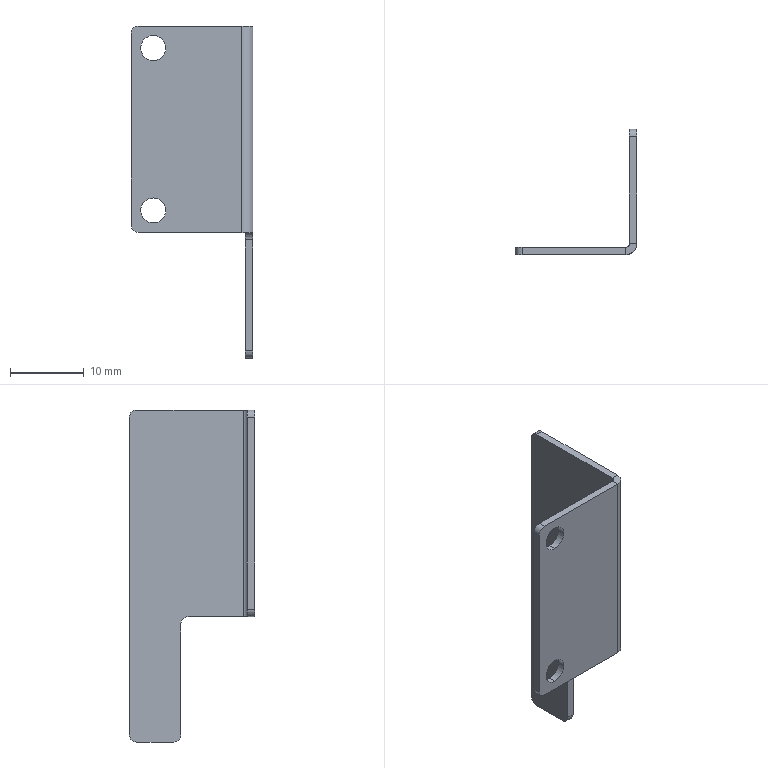Part | NX | features BREP 1 | 1 solid | 26 faces | box 16.5 x 17 x 45 mm | volume 997.965 mm3 | plane 14 | cylinder 12 | commonest cylinder face diameters 2 x6 3.4 x4 1 x1 3 x1
STEP:
#1=CARTESIAN_POINT('',(-12.5,-16.,17.8));
#2=VERTEX_POINT('',#1);
#3=CARTESIAN_POINT('',(-12.5,-17.,17.8));
#4=VERTEX_POINT('',#3);
#5=CARTESIAN_POINT('',(-12.5,-16.,17.8));
#6=DIRECTION('',(0.,1.,0.));
#7=VECTOR('',#6,1000.);
#8=LINE('',#5,#7);
#9=EDGE_CURVE('',#2,#4,#8,.F.);
#10=ORIENTED_EDGE('',*,*,#9,.T.);
#11=CARTESIAN_POINT('',(-12.5,-17.,21.2));
#12=VERTEX_POINT('',#11);
#13=CARTESIAN_POINT('',(-12.5,-17.,19.5));
#14=DIRECTION('',(0.,1.,0.));
#15=DIRECTION('',(0.,0.,1.));
#16=AXIS2_PLACEMENT_3D('',#13,#14,#15);
#17=CIRCLE('',#16,1.7);
#18=EDGE_CURVE('',#12,#4,#17,.T.);
#19=ORIENTED_EDGE('',*,*,#18,.F.);
#20=CARTESIAN_POINT('',(-12.5,-16.,21.2));
#21=VERTEX_POINT('',#20);
#22=CARTESIAN_POINT('',(-12.5,-16.,21.2));
#23=DIRECTION('',(0.,1.,0.));
#24=VECTOR('',#23,1000.);
#25=LINE('',#22,#24);
#26=EDGE_CURVE('',#21,#12,#25,.F.);
#27=ORIENTED_EDGE('',*,*,#26,.F.);
#28=CARTESIAN_POINT('',(-12.5,-16.,19.5));
#29=DIRECTION('',(0.,1.,0.));
#30=DIRECTION('',(0.,0.,1.));
#31=AXIS2_PLACEMENT_3D('',#28,#29,#30);
#32=CIRCLE('',#31,1.7);
#33=EDGE_CURVE('',#21,#2,#32,.T.);
#34=ORIENTED_EDGE('',*,*,#33,.T.);
#35=EDGE_LOOP('',(#10,#19,#27,#34));
#36=FACE_BOUND('',#35,.T.);
#37=CARTESIAN_POINT('',(-12.5,-16.,19.5));
#38=DIRECTION('',(0.,1.,0.));
#39=DIRECTION('',(0.,0.,1.));
#40=AXIS2_PLACEMENT_3D('',#37,#38,#39);
#41=CYLINDRICAL_SURFACE('',#40,1.7);
#42=ADVANCED_FACE('',(#36),#41,.F.);
#43=CARTESIAN_POINT('',(-12.5,-16.,-4.2));
#44=VERTEX_POINT('',#43);
#45=CARTESIAN_POINT('',(-12.5,-17.,-4.2));
#46=VERTEX_POINT('',#45);
#47=CARTESIAN_POINT('',(-12.5,-16.,-4.2));
#48=DIRECTION('',(0.,1.,0.));
#49=VECTOR('',#48,1000.);
#50=LINE('',#47,#49);
#51=EDGE_CURVE('',#44,#46,#50,.F.);
#52=ORIENTED_EDGE('',*,*,#51,.T.);
#53=CARTESIAN_POINT('',(-12.5,-17.,-0.8));
#54=VERTEX_POINT('',#53);
#55=CARTESIAN_POINT('',(-12.5,-17.,-2.5));
#56=DIRECTION('',(0.,1.,0.));
#57=DIRECTION('',(0.,0.,1.));
#58=AXIS2_PLACEMENT_3D('',#55,#56,#57);
#59=CIRCLE('',#58,1.7);
#60=EDGE_CURVE('',#54,#46,#59,.T.);
#61=ORIENTED_EDGE('',*,*,#60,.F.);
#62=CARTESIAN_POINT('',(-12.5,-16.,-0.8));
#63=VERTEX_POINT('',#62);
#64=CARTESIAN_POINT('',(-12.5,-16.,-0.8));
#65=DIRECTION('',(0.,1.,0.));
#66=VECTOR('',#65,1000.);
#67=LINE('',#64,#66);
#68=EDGE_CURVE('',#63,#54,#67,.F.);
#69=ORIENTED_EDGE('',*,*,#68,.F.);
#70=CARTESIAN_POINT('',(-12.5,-16.,-2.5));
#71=DIRECTION('',(0.,1.,0.));
#72=DIRECTION('',(0.,0.,1.));
#73=AXIS2_PLACEMENT_3D('',#70,#71,#72);
#74=CIRCLE('',#73,1.7);
#75=EDGE_CURVE('',#63,#44,#74,.T.);
#76=ORIENTED_EDGE('',*,*,#75,.T.);
#77=EDGE_LOOP('',(#52,#61,#69,#76));
#78=FACE_BOUND('',#77,.T.);
#79=CARTESIAN_POINT('',(-12.5,-16.,-2.5));
#80=DIRECTION('',(0.,1.,0.));
#81=DIRECTION('',(0.,0.,1.));
#82=AXIS2_PLACEMENT_3D('',#79,#80,#81);
#83=CYLINDRICAL_SURFACE('',#82,1.7);
#84=ADVANCED_FACE('',(#78),#83,.F.);
#85=CARTESIAN_POINT('',(-14.5,-17.,22.5));
#86=VERTEX_POINT('',#85);
#87=CARTESIAN_POINT('',(-15.5,-17.,21.5));
#88=VERTEX_POINT('',#87);
#89=CARTESIAN_POINT('',(-14.5,-17.,21.5));
#90=DIRECTION('',(0.,-1.,0.));
#91=DIRECTION('',(-1.,0.,0.));
#92=AXIS2_PLACEMENT_3D('',#89,#90,#91);
#93=CIRCLE('',#92,1.);
#94=EDGE_CURVE('',#86,#88,#93,.T.);
#95=ORIENTED_EDGE('',*,*,#94,.F.);
#96=CARTESIAN_POINT('',(-14.5,-16.,22.5));
#97=VERTEX_POINT('',#96);
#98=CARTESIAN_POINT('',(-14.5,-15.5,22.5));
#99=DIRECTION('',(0.,-1.,0.));
#100=VECTOR('',#99,1000.);
#101=LINE('',#98,#100);
#102=EDGE_CURVE('',#97,#86,#101,.T.);
#103=ORIENTED_EDGE('',*,*,#102,.F.);
#104=CARTESIAN_POINT('',(-15.5,-16.,21.5));
#105=VERTEX_POINT('',#104);
#106=CARTESIAN_POINT('',(-14.5,-16.,21.5));
#107=DIRECTION('',(0.,1.,0.));
#108=DIRECTION('',(-1.,0.,0.));
#109=AXIS2_PLACEMENT_3D('',#106,#107,#108);
#110=CIRCLE('',#109,1.);
#111=EDGE_CURVE('',#105,#97,#110,.T.);
#112=ORIENTED_EDGE('',*,*,#111,.F.);
#113=CARTESIAN_POINT('',(-15.5,-17.,21.5));
#114=DIRECTION('',(0.,1.,0.));
#115=VECTOR('',#114,1000.);
#116=LINE('',#113,#115);
#117=EDGE_CURVE('',#88,#105,#116,.T.);
#118=ORIENTED_EDGE('',*,*,#117,.F.);
#119=EDGE_LOOP('',(#95,#103,#112,#118));
#120=FACE_BOUND('',#119,.T.);
#121=CARTESIAN_POINT('',(-14.5,-17.,21.5));
#122=DIRECTION('',(0.,1.,0.));
#123=DIRECTION('',(0.,0.,1.));
#124=AXIS2_PLACEMENT_3D('',#121,#122,#123);
#125=CYLINDRICAL_SURFACE('',#124,1.);
#126=ADVANCED_FACE('',(#120),#125,.T.);
#127=CARTESIAN_POINT('',(-14.5,-16.,-5.5));
#128=VERTEX_POINT('',#127);
#129=CARTESIAN_POINT('',(-15.5,-16.,-4.5));
#130=VERTEX_POINT('',#129);
#131=CARTESIAN_POINT('',(-14.5,-16.,-4.5));
#132=DIRECTION('',(0.,1.,0.));
#133=DIRECTION('',(-1.,0.,0.));
#134=AXIS2_PLACEMENT_3D('',#131,#132,#133);
#135=CIRCLE('',#134,1.);
#136=EDGE_CURVE('',#128,#130,#135,.T.);
#137=ORIENTED_EDGE('',*,*,#136,.F.);
#138=CARTESIAN_POINT('',(-14.5,-17.,-5.5));
#139=VERTEX_POINT('',#138);
#140=CARTESIAN_POINT('',(-14.5,-16.,-5.5));
#141=DIRECTION('',(0.,1.,0.));
#142=VECTOR('',#141,1000.);
#143=LINE('',#140,#142);
#144=EDGE_CURVE('',#139,#128,#143,.T.);
#145=ORIENTED_EDGE('',*,*,#144,.F.);
#146=CARTESIAN_POINT('',(-15.5,-17.,-4.5));
#147=VERTEX_POINT('',#146);
#148=CARTESIAN_POINT('',(-14.5,-17.,-4.5));
#149=DIRECTION('',(0.,-1.,0.));
#150=DIRECTION('',(-1.,0.,0.));
#151=AXIS2_PLACEMENT_3D('',#148,#149,#150);
#152=CIRCLE('',#151,1.);
#153=EDGE_CURVE('',#147,#139,#152,.T.);
#154=ORIENTED_EDGE('',*,*,#153,.F.);
#155=CARTESIAN_POINT('',(-15.5,-17.,-4.5));
#156=DIRECTION('',(0.,-1.,0.));
#157=VECTOR('',#156,1000.);
#158=LINE('',#155,#157);
#159=EDGE_CURVE('',#130,#147,#158,.T.);
#160=ORIENTED_EDGE('',*,*,#159,.F.);
#161=EDGE_LOOP('',(#137,#145,#154,#160));
#162=FACE_BOUND('',#161,.T.);
#163=CARTESIAN_POINT('',(-14.5,-17.,-4.5));
#164=DIRECTION('',(0.,1.,0.));
#165=DIRECTION('',(0.,0.,1.));
#166=AXIS2_PLACEMENT_3D('',#163,#164,#165);
#167=CYLINDRICAL_SURFACE('',#166,1.);
#168=ADVANCED_FACE('',(#162),#167,.T.);
#169=CARTESIAN_POINT('',(0.,-1.,22.5));
#170=VERTEX_POINT('',#169);
#171=CARTESIAN_POINT('',(0.,0.,21.5));
#172=VERTEX_POINT('',#171);
#173=CARTESIAN_POINT('',(0.,-1.,21.5));
#174=DIRECTION('',(-1.,0.,0.));
#175=DIRECTION('',(0.,-1.,0.));
#176=AXIS2_PLACEMENT_3D('',#173,#174,#175);
#177=CIRCLE('',#176,1.);
#178=EDGE_CURVE('',#170,#172,#177,.T.);
#179=ORIENTED_EDGE('',*,*,#178,.F.);
#180=CARTESIAN_POINT('',(1.,-1.,22.5));
#181=VERTEX_POINT('',#180);
#182=CARTESIAN_POINT('',(-0.5,-1.,22.5));
#183=DIRECTION('',(-1.,0.,0.));
#184=VECTOR('',#183,1000.);
#185=LINE('',#182,#184);
#186=EDGE_CURVE('',#181,#170,#185,.T.);
#187=ORIENTED_EDGE('',*,*,#186,.F.);
#188=CARTESIAN_POINT('',(1.,0.,21.5));
#189=VERTEX_POINT('',#188);
#190=CARTESIAN_POINT('',(1.,-1.,21.5));
#191=DIRECTION('',(1.,0.,0.));
#192=DIRECTION('',(0.,-1.,0.));
#193=AXIS2_PLACEMENT_3D('',#190,#191,#192);
#194=CIRCLE('',#193,1.);
#195=EDGE_CURVE('',#189,#181,#194,.T.);
#196=ORIENTED_EDGE('',*,*,#195,.F.);
#197=CARTESIAN_POINT('',(0.,0.,21.5));
#198=DIRECTION('',(1.,0.,0.));
#199=VECTOR('',#198,1000.);
#200=LINE('',#197,#199);
#201=EDGE_CURVE('',#172,#189,#200,.T.);
#202=ORIENTED_EDGE('',*,*,#201,.F.);
#203=EDGE_LOOP('',(#179,#187,#196,#202));
#204=FACE_BOUND('',#203,.T.);
#205=CARTESIAN_POINT('',(0.,-1.,21.5));
#206=DIRECTION('',(1.,0.,0.));
#207=DIRECTION('',(0.,1.,0.));
#208=AXIS2_PLACEMENT_3D('',#205,#206,#207);
#209=CYLINDRICAL_SURFACE('',#208,1.);
#210=ADVANCED_FACE('',(#204),#209,.T.);
#211=CARTESIAN_POINT('',(0.,-7.,-6.5));
#212=VERTEX_POINT('',#211);
#213=CARTESIAN_POINT('',(0.,-8.,-5.5));
#214=VERTEX_POINT('',#213);
#215=CARTESIAN_POINT('',(0.,-8.,-6.5));
#216=DIRECTION('',(1.,0.,0.));
#217=DIRECTION('',(0.,-1.,0.));
#218=AXIS2_PLACEMENT_3D('',#215,#216,#217);
#219=CIRCLE('',#218,1.);
#220=EDGE_CURVE('',#212,#214,#219,.T.);
#221=ORIENTED_EDGE('',*,*,#220,.F.);
#222=CARTESIAN_POINT('',(1.,-7.,-6.5));
#223=VERTEX_POINT('',#222);
#224=CARTESIAN_POINT('',(0.,-7.,-6.5));
#225=DIRECTION('',(-1.,0.,0.));
#226=VECTOR('',#225,1000.);
#227=LINE('',#224,#226);
#228=EDGE_CURVE('',#223,#212,#227,.T.);
#229=ORIENTED_EDGE('',*,*,#228,.F.);
#230=CARTESIAN_POINT('',(1.,-8.,-5.5));
#231=VERTEX_POINT('',#230);
#232=CARTESIAN_POINT('',(1.,-8.,-6.5));
#233=DIRECTION('',(-1.,0.,0.));
#234=DIRECTION('',(0.,-1.,0.));
#235=AXIS2_PLACEMENT_3D('',#232,#233,#234);
#236=CIRCLE('',#235,1.);
#237=EDGE_CURVE('',#231,#223,#236,.T.);
#238=ORIENTED_EDGE('',*,*,#237,.F.);
#239=CARTESIAN_POINT('',(1.,-8.,-5.5));
#240=DIRECTION('',(1.,0.,0.));
#241=VECTOR('',#240,1000.);
#242=LINE('',#239,#241);
#243=EDGE_CURVE('',#214,#231,#242,.T.);
#244=ORIENTED_EDGE('',*,*,#243,.F.);
#245=EDGE_LOOP('',(#221,#229,#238,#244));
#246=FACE_BOUND('',#245,.T.);
#247=CARTESIAN_POINT('',(-15.5,-8.,-6.5));
#248=DIRECTION('',(-1.,0.,0.));
#249=DIRECTION('',(0.,-1.,0.));
#250=AXIS2_PLACEMENT_3D('',#247,#248,#249);
#251=CYLINDRICAL_SURFACE('',#250,1.);
#252=ADVANCED_FACE('',(#246),#251,.F.);
#253=CARTESIAN_POINT('',(0.,0.,-21.5));
#254=VERTEX_POINT('',#253);
#255=CARTESIAN_POINT('',(0.,-1.,-22.5));
#256=VERTEX_POINT('',#255);
#257=CARTESIAN_POINT('',(0.,-1.,-21.5));
#258=DIRECTION('',(-1.,0.,0.));
#259=DIRECTION('',(0.,-1.,0.));
#260=AXIS2_PLACEMENT_3D('',#257,#258,#259);
#261=CIRCLE('',#260,1.);
#262=EDGE_CURVE('',#254,#256,#261,.T.);
#263=ORIENTED_EDGE('',*,*,#262,.F.);
#264=CARTESIAN_POINT('',(1.,0.,-21.5));
#265=VERTEX_POINT('',#264);
#266=CARTESIAN_POINT('',(0.,0.,-21.5));
#267=DIRECTION('',(-1.,0.,0.));
#268=VECTOR('',#267,1000.);
#269=LINE('',#266,#268);
#270=EDGE_CURVE('',#265,#254,#269,.T.);
#271=ORIENTED_EDGE('',*,*,#270,.F.);
#272=CARTESIAN_POINT('',(1.,-1.,-22.5));
#273=VERTEX_POINT('',#272);
#274=CARTESIAN_POINT('',(1.,-1.,-21.5));
#275=DIRECTION('',(1.,0.,0.));
#276=DIRECTION('',(0.,-1.,0.));
#277=AXIS2_PLACEMENT_3D('',#274,#275,#276);
#278=CIRCLE('',#277,1.);
#279=EDGE_CURVE('',#273,#265,#278,.T.);
#280=ORIENTED_EDGE('',*,*,#279,.F.);
#281=CARTESIAN_POINT('',(1.,-1.,-22.5));
#282=DIRECTION('',(1.,0.,0.));
#283=VECTOR('',#282,1000.);
#284=LINE('',#281,#283);
#285=EDGE_CURVE('',#256,#273,#284,.T.);
#286=ORIENTED_EDGE('',*,*,#285,.F.);
#287=EDGE_LOOP('',(#263,#271,#280,#286));
#288=FACE_BOUND('',#287,.T.);
#289=CARTESIAN_POINT('',(-0.5,-1.,-21.5));
#290=DIRECTION('',(-1.,0.,0.));
#291=DIRECTION('',(0.,-1.,0.));
#292=AXIS2_PLACEMENT_3D('',#289,#290,#291);
#293=CYLINDRICAL_SURFACE('',#292,1.);
#294=ADVANCED_FACE('',(#288),#293,.T.);
#295=CARTESIAN_POINT('',(1.,-7.,-21.5));
#296=VERTEX_POINT('',#295);
#297=CARTESIAN_POINT('',(1.,-6.,-22.5));
#298=VERTEX_POINT('',#297);
#299=CARTESIAN_POINT('',(1.,-6.,-21.5));
#300=DIRECTION('',(1.,0.,0.));
#301=DIRECTION('',(0.,-1.,0.));
#302=AXIS2_PLACEMENT_3D('',#299,#300,#301);
#303=CIRCLE('',#302,1.);
#304=EDGE_CURVE('',#296,#298,#303,.T.);
#305=ORIENTED_EDGE('',*,*,#304,.F.);
#306=CARTESIAN_POINT('',(0.,-7.,-21.5));
#307=VERTEX_POINT('',#306);
#308=CARTESIAN_POINT('',(-15.5,-7.,-21.5));
#309=DIRECTION('',(1.,0.,0.));
#310=VECTOR('',#309,1000.);
#311=LINE('',#308,#310);
#312=EDGE_CURVE('',#307,#296,#311,.T.);
#313=ORIENTED_EDGE('',*,*,#312,.F.);
#314=CARTESIAN_POINT('',(0.,-6.,-22.5));
#315=VERTEX_POINT('',#314);
#316=CARTESIAN_POINT('',(0.,-6.,-21.5));
#317=DIRECTION('',(-1.,0.,0.));
#318=DIRECTION('',(0.,-1.,0.));
#319=AXIS2_PLACEMENT_3D('',#316,#317,#318);
#320=CIRCLE('',#319,1.);
#321=EDGE_CURVE('',#315,#307,#320,.T.);
#322=ORIENTED_EDGE('',*,*,#321,.F.);
#323=CARTESIAN_POINT('',(-0.5,-6.,-22.5));
#324=DIRECTION('',(-1.,0.,0.));
#325=VECTOR('',#324,1000.);
#326=LINE('',#323,#325);
#327=EDGE_CURVE('',#298,#315,#326,.T.);
#328=ORIENTED_EDGE('',*,*,#327,.F.);
#329=EDGE_LOOP('',(#305,#313,#322,#328));
#330=FACE_BOUND('',#329,.T.);
#331=CARTESIAN_POINT('',(-0.5,-6.,-21.5));
#332=DIRECTION('',(-1.,0.,0.));
#333=DIRECTION('',(0.,-1.,0.));
#334=AXIS2_PLACEMENT_3D('',#331,#332,#333);
#335=CYLINDRICAL_SURFACE('',#334,1.);
#336=ADVANCED_FACE('',(#330),#335,.T.);
#337=CARTESIAN_POINT('',(0.,-7.,22.5));
#338=DIRECTION('',(0.,0.,-1.));
#339=VECTOR('',#338,1000.);
#340=LINE('',#337,#339);
#341=EDGE_CURVE('',#212,#307,#340,.T.);
#342=ORIENTED_EDGE('',*,*,#341,.T.);
#343=ORIENTED_EDGE('',*,*,#312,.T.);
#344=CARTESIAN_POINT('',(1.,-7.,-22.5));
#345=DIRECTION('',(0.,0.,1.));
#346=VECTOR('',#345,1000.);
#347=LINE('',#344,#346);
#348=EDGE_CURVE('',#296,#223,#347,.T.);
#349=ORIENTED_EDGE('',*,*,#348,.T.);
#350=ORIENTED_EDGE('',*,*,#228,.T.);
#351=EDGE_LOOP('',(#342,#343,#349,#350));
#352=FACE_BOUND('',#351,.T.);
#353=CARTESIAN_POINT('',(-15.5,-7.,-22.5));
#354=DIRECTION('',(0.,1.,0.));
#355=DIRECTION('',(-1.,0.,0.));
#356=AXIS2_PLACEMENT_3D('',#353,#354,#355);
#357=PLANE('',#356);
#358=ADVANCED_FACE('',(#352),#357,.F.);
#359=CARTESIAN_POINT('',(-0.5,-16.,-5.5));
#360=VERTEX_POINT('',#359);
#361=CARTESIAN_POINT('',(-0.5,-17.,-5.5));
#362=VERTEX_POINT('',#361);
#363=CARTESIAN_POINT('',(-0.5,-16.,-5.5));
#364=DIRECTION('',(0.,-1.,0.));
#365=VECTOR('',#364,1000.);
#366=LINE('',#363,#365);
#367=EDGE_CURVE('',#360,#362,#366,.T.);
#368=ORIENTED_EDGE('',*,*,#367,.F.);
#369=CARTESIAN_POINT('',(0.,-15.5,-5.5));
#370=VERTEX_POINT('',#369);
#371=CARTESIAN_POINT('',(-0.5,-15.5,-5.5));
#372=DIRECTION('',(0.,0.,1.));
#373=DIRECTION('',(1.,0.,0.));
#374=AXIS2_PLACEMENT_3D('',#371,#372,#373);
#375=CIRCLE('',#374,0.5);
#376=EDGE_CURVE('',#360,#370,#375,.T.);
#377=ORIENTED_EDGE('',*,*,#376,.T.);
#378=CARTESIAN_POINT('',(1.,-15.5,-5.5));
#379=VERTEX_POINT('',#378);
#380=CARTESIAN_POINT('',(1.,-15.5,-5.5));
#381=DIRECTION('',(-1.,0.,0.));
#382=VECTOR('',#381,1000.);
#383=LINE('',#380,#382);
#384=EDGE_CURVE('',#379,#370,#383,.T.);
#385=ORIENTED_EDGE('',*,*,#384,.F.);
#386=CARTESIAN_POINT('',(-0.5,-15.5,-5.5));
#387=DIRECTION('',(0.,0.,1.));
#388=DIRECTION('',(1.,0.,0.));
#389=AXIS2_PLACEMENT_3D('',#386,#387,#388);
#390=CIRCLE('',#389,1.5);
#391=EDGE_CURVE('',#362,#379,#390,.T.);
#392=ORIENTED_EDGE('',*,*,#391,.F.);
#393=EDGE_LOOP('',(#368,#377,#385,#392));
#394=FACE_BOUND('',#393,.T.);
#395=CARTESIAN_POINT('',(-15.5,-17.,-5.5));
#396=DIRECTION('',(0.,0.,1.));
#397=DIRECTION('',(1.,0.,0.));
#398=AXIS2_PLACEMENT_3D('',#395,#396,#397);
#399=PLANE('',#398);
#400=ADVANCED_FACE('',(#394),#399,.F.);
#401=CARTESIAN_POINT('',(1.,0.,-22.5));
#402=DIRECTION('',(0.,1.,0.));
#403=VECTOR('',#402,1000.);
#404=LINE('',#401,#403);
#405=EDGE_CURVE('',#298,#273,#404,.T.);
#406=ORIENTED_EDGE('',*,*,#405,.F.);
#407=ORIENTED_EDGE('',*,*,#327,.T.);
#408=CARTESIAN_POINT('',(0.,0.,-22.5));
#409=DIRECTION('',(0.,1.,0.));
#410=VECTOR('',#409,1000.);
#411=LINE('',#408,#410);
#412=EDGE_CURVE('',#315,#256,#411,.T.);
#413=ORIENTED_EDGE('',*,*,#412,.T.);
#414=ORIENTED_EDGE('',*,*,#285,.T.);
#415=EDGE_LOOP('',(#406,#407,#413,#414));
#416=FACE_BOUND('',#415,.T.);
#417=CARTESIAN_POINT('',(-0.5,-15.5,-22.5));
#418=DIRECTION('',(0.,0.,1.));
#419=DIRECTION('',(1.,0.,0.));
#420=AXIS2_PLACEMENT_3D('',#417,#418,#419);
#421=PLANE('',#420);
#422=ADVANCED_FACE('',(#416),#421,.F.);
#423=CARTESIAN_POINT('',(-0.5,-16.,22.5));
#424=VERTEX_POINT('',#423);
#425=CARTESIAN_POINT('',(0.,-16.,22.5));
#426=DIRECTION('',(1.,0.,0.));
#427=VECTOR('',#426,1000.);
#428=LINE('',#425,#427);
#429=EDGE_CURVE('',#97,#424,#428,.T.);
#430=ORIENTED_EDGE('',*,*,#429,.F.);
#431=ORIENTED_EDGE('',*,*,#102,.T.);
#432=CARTESIAN_POINT('',(-0.5,-17.,22.5));
#433=VERTEX_POINT('',#432);
#434=CARTESIAN_POINT('',(0.,-17.,22.5));
#435=DIRECTION('',(1.,0.,0.));
#436=VECTOR('',#435,1000.);
#437=LINE('',#434,#436);
#438=EDGE_CURVE('',#86,#433,#437,.T.);
#439=ORIENTED_EDGE('',*,*,#438,.T.);
#440=CARTESIAN_POINT('',(-0.5,-17.,22.5));
#441=DIRECTION('',(0.,1.,0.));
#442=VECTOR('',#441,1000.);
#443=LINE('',#440,#442);
#444=EDGE_CURVE('',#433,#424,#443,.T.);
#445=ORIENTED_EDGE('',*,*,#444,.T.);
#446=EDGE_LOOP('',(#430,#431,#439,#445));
#447=FACE_BOUND('',#446,.T.);
#448=CARTESIAN_POINT('',(-0.5,-15.5,22.5));
#449=DIRECTION('',(0.,0.,1.));
#450=DIRECTION('',(1.,0.,0.));
#451=AXIS2_PLACEMENT_3D('',#448,#449,#450);
#452=PLANE('',#451);
#453=ADVANCED_FACE('',(#447),#452,.T.);
#454=CARTESIAN_POINT('',(-0.5,-17.,22.5));
#455=DIRECTION('',(0.,0.,-1.));
#456=VECTOR('',#455,1000.);
#457=LINE('',#454,#456);
#458=EDGE_CURVE('',#433,#362,#457,.T.);
#459=ORIENTED_EDGE('',*,*,#458,.T.);
#460=ORIENTED_EDGE('',*,*,#391,.T.);
#461=CARTESIAN_POINT('',(1.,-15.5,22.5));
#462=VERTEX_POINT('',#461);
#463=CARTESIAN_POINT('',(1.,-15.5,22.5));
#464=DIRECTION('',(0.,0.,-1.));
#465=VECTOR('',#464,1000.);
#466=LINE('',#463,#465);
#467=EDGE_CURVE('',#462,#379,#466,.T.);
#468=ORIENTED_EDGE('',*,*,#467,.F.);
#469=CARTESIAN_POINT('',(-0.5,-15.5,22.5));
#470=DIRECTION('',(0.,0.,1.));
#471=DIRECTION('',(1.,0.,0.));
#472=AXIS2_PLACEMENT_3D('',#469,#470,#471);
#473=CIRCLE('',#472,1.5);
#474=EDGE_CURVE('',#433,#462,#473,.T.);
#475=ORIENTED_EDGE('',*,*,#474,.F.);
#476=EDGE_LOOP('',(#459,#460,#468,#475));
#477=FACE_BOUND('',#476,.T.);
#478=CARTESIAN_POINT('',(-0.5,-15.5,22.5));
#479=DIRECTION('',(0.,0.,-1.));
#480=DIRECTION('',(-1.,0.,0.));
#481=AXIS2_PLACEMENT_3D('',#478,#479,#480);
#482=CYLINDRICAL_SURFACE('',#481,1.5);
#483=ADVANCED_FACE('',(#477),#482,.T.);
#484=CARTESIAN_POINT('',(-15.5,-17.,22.5));
#485=DIRECTION('',(0.,0.,-1.));
#486=VECTOR('',#485,1000.);
#487=LINE('',#484,#486);
#488=EDGE_CURVE('',#88,#147,#487,.T.);
#489=ORIENTED_EDGE('',*,*,#488,.T.);
#490=ORIENTED_EDGE('',*,*,#153,.T.);
#491=CARTESIAN_POINT('',(-15.5,-17.,-5.5));
#492=DIRECTION('',(1.,0.,0.));
#493=VECTOR('',#492,1000.);
#494=LINE('',#491,#493);
#495=EDGE_CURVE('',#139,#362,#494,.T.);
#496=ORIENTED_EDGE('',*,*,#495,.T.);
#497=ORIENTED_EDGE('',*,*,#458,.F.);
#498=ORIENTED_EDGE('',*,*,#438,.F.);
#499=ORIENTED_EDGE('',*,*,#94,.T.);
#500=EDGE_LOOP('',(#489,#490,#496,#497,#498,#499));
#501=FACE_BOUND('',#500,.T.);
#502=ORIENTED_EDGE('',*,*,#60,.T.);
#503=CARTESIAN_POINT('',(-12.5,-17.,-2.5));
#504=DIRECTION('',(0.,1.,0.));
#505=DIRECTION('',(0.,0.,1.));
#506=AXIS2_PLACEMENT_3D('',#503,#504,#505);
#507=CIRCLE('',#506,1.7);
#508=EDGE_CURVE('',#46,#54,#507,.T.);
#509=ORIENTED_EDGE('',*,*,#508,.T.);
#510=EDGE_LOOP('',(#502,#509));
#511=FACE_BOUND('',#510,.T.);
#512=ORIENTED_EDGE('',*,*,#18,.T.);
#513=CARTESIAN_POINT('',(-12.5,-17.,19.5));
#514=DIRECTION('',(0.,1.,0.));
#515=DIRECTION('',(0.,0.,1.));
#516=AXIS2_PLACEMENT_3D('',#513,#514,#515);
#517=CIRCLE('',#516,1.7);
#518=EDGE_CURVE('',#4,#12,#517,.T.);
#519=ORIENTED_EDGE('',*,*,#518,.T.);
#520=EDGE_LOOP('',(#512,#519));
#521=FACE_BOUND('',#520,.T.);
#522=CARTESIAN_POINT('',(0.,-17.,22.5));
#523=DIRECTION('',(0.,1.,0.));
#524=DIRECTION('',(-1.,0.,0.));
#525=AXIS2_PLACEMENT_3D('',#522,#523,#524);
#526=PLANE('',#525);
#527=ADVANCED_FACE('',(#501,#511,#521),#526,.F.);
#528=CARTESIAN_POINT('',(-15.5,-16.,22.5));
#529=DIRECTION('',(0.,0.,-1.));
#530=VECTOR('',#529,1000.);
#531=LINE('',#528,#530);
#532=EDGE_CURVE('',#105,#130,#531,.T.);
#533=ORIENTED_EDGE('',*,*,#532,.T.);
#534=ORIENTED_EDGE('',*,*,#159,.T.);
#535=ORIENTED_EDGE('',*,*,#488,.F.);
#536=ORIENTED_EDGE('',*,*,#117,.T.);
#537=EDGE_LOOP('',(#533,#534,#535,#536));
#538=FACE_BOUND('',#537,.T.);
#539=CARTESIAN_POINT('',(-15.5,-17.,22.5));
#540=DIRECTION('',(-1.,0.,0.));
#541=DIRECTION('',(0.,0.,1.));
#542=AXIS2_PLACEMENT_3D('',#539,#540,#541);
#543=PLANE('',#542);
#544=ADVANCED_FACE('',(#538),#543,.T.);
#545=CARTESIAN_POINT('',(0.,-16.,-5.5));
#546=DIRECTION('',(1.,0.,0.));
#547=VECTOR('',#546,1000.);
#548=LINE('',#545,#547);
#549=EDGE_CURVE('',#128,#360,#548,.T.);
#550=ORIENTED_EDGE('',*,*,#549,.F.);
#551=ORIENTED_EDGE('',*,*,#136,.T.);
#552=ORIENTED_EDGE('',*,*,#532,.F.);
#553=ORIENTED_EDGE('',*,*,#111,.T.);
#554=ORIENTED_EDGE('',*,*,#429,.T.);
#555=CARTESIAN_POINT('',(-0.5,-16.,22.5));
#556=DIRECTION('',(0.,0.,-1.));
#557=VECTOR('',#556,1000.);
#558=LINE('',#555,#557);
#559=EDGE_CURVE('',#424,#360,#558,.T.);
#560=ORIENTED_EDGE('',*,*,#559,.T.);
#561=EDGE_LOOP('',(#550,#551,#552,#553,#554,#560));
#562=FACE_BOUND('',#561,.T.);
#563=ORIENTED_EDGE('',*,*,#75,.F.);
#564=CARTESIAN_POINT('',(-12.5,-16.,-2.5));
#565=DIRECTION('',(0.,1.,0.));
#566=DIRECTION('',(0.,0.,1.));
#567=AXIS2_PLACEMENT_3D('',#564,#565,#566);
#568=CIRCLE('',#567,1.7);
#569=EDGE_CURVE('',#44,#63,#568,.T.);
#570=ORIENTED_EDGE('',*,*,#569,.F.);
#571=EDGE_LOOP('',(#563,#570));
#572=FACE_BOUND('',#571,.T.);
#573=ORIENTED_EDGE('',*,*,#33,.F.);
#574=CARTESIAN_POINT('',(-12.5,-16.,19.5));
#575=DIRECTION('',(0.,1.,0.));
#576=DIRECTION('',(0.,0.,1.));
#577=AXIS2_PLACEMENT_3D('',#574,#575,#576);
#578=CIRCLE('',#577,1.7);
#579=EDGE_CURVE('',#2,#21,#578,.T.);
#580=ORIENTED_EDGE('',*,*,#579,.F.);
#581=EDGE_LOOP('',(#573,#580));
#582=FACE_BOUND('',#581,.T.);
#583=CARTESIAN_POINT('',(0.,-16.,22.5));
#584=DIRECTION('',(0.,1.,0.));
#585=DIRECTION('',(-1.,0.,0.));
#586=AXIS2_PLACEMENT_3D('',#583,#584,#585);
#587=PLANE('',#586);
#588=ADVANCED_FACE('',(#562,#572,#582),#587,.T.);
#589=ORIENTED_EDGE('',*,*,#376,.F.);
#590=ORIENTED_EDGE('',*,*,#559,.F.);
#591=CARTESIAN_POINT('',(0.,-15.5,22.5));
#592=VERTEX_POINT('',#591);
#593=CARTESIAN_POINT('',(-0.5,-15.5,22.5));
#594=DIRECTION('',(0.,0.,1.));
#595=DIRECTION('',(1.,0.,0.));
#596=AXIS2_PLACEMENT_3D('',#593,#594,#595);
#597=CIRCLE('',#596,0.5);
#598=EDGE_CURVE('',#424,#592,#597,.T.);
#599=ORIENTED_EDGE('',*,*,#598,.T.);
#600=CARTESIAN_POINT('',(0.,-15.5,22.5));
#601=DIRECTION('',(0.,0.,-1.));
#602=VECTOR('',#601,1000.);
#603=LINE('',#600,#602);
#604=EDGE_CURVE('',#592,#370,#603,.T.);
#605=ORIENTED_EDGE('',*,*,#604,.T.);
#606=EDGE_LOOP('',(#589,#590,#599,#605));
#607=FACE_BOUND('',#606,.T.);
#608=CARTESIAN_POINT('',(-0.5,-15.5,22.5));
#609=DIRECTION('',(0.,0.,-1.));
#610=DIRECTION('',(-1.,0.,0.));
#611=AXIS2_PLACEMENT_3D('',#608,#609,#610);
#612=CYLINDRICAL_SURFACE('',#611,0.5);
#613=ADVANCED_FACE('',(#607),#612,.F.);
#614=ORIENTED_EDGE('',*,*,#412,.F.);
#615=ORIENTED_EDGE('',*,*,#321,.T.);
#616=ORIENTED_EDGE('',*,*,#341,.F.);
#617=ORIENTED_EDGE('',*,*,#220,.T.);
#618=CARTESIAN_POINT('',(0.,0.,-5.5));
#619=DIRECTION('',(0.,1.,0.));
#620=VECTOR('',#619,1000.);
#621=LINE('',#618,#620);
#622=EDGE_CURVE('',#370,#214,#621,.T.);
#623=ORIENTED_EDGE('',*,*,#622,.F.);
#624=ORIENTED_EDGE('',*,*,#604,.F.);
#625=CARTESIAN_POINT('',(0.,0.,22.5));
#626=DIRECTION('',(0.,1.,0.));
#627=VECTOR('',#626,1000.);
#628=LINE('',#625,#627);
#629=EDGE_CURVE('',#592,#170,#628,.T.);
#630=ORIENTED_EDGE('',*,*,#629,.T.);
#631=ORIENTED_EDGE('',*,*,#178,.T.);
#632=CARTESIAN_POINT('',(0.,0.,22.5));
#633=DIRECTION('',(0.,0.,-1.));
#634=VECTOR('',#633,1000.);
#635=LINE('',#632,#634);
#636=EDGE_CURVE('',#172,#254,#635,.T.);
#637=ORIENTED_EDGE('',*,*,#636,.T.);
#638=ORIENTED_EDGE('',*,*,#262,.T.);
#639=EDGE_LOOP('',(#614,#615,#616,#617,#623,#624,#630,#631,#637,#638));
#640=FACE_BOUND('',#639,.T.);
#641=CARTESIAN_POINT('',(0.,0.,22.5));
#642=DIRECTION('',(-1.,0.,0.));
#643=DIRECTION('',(0.,-1.,0.));
#644=AXIS2_PLACEMENT_3D('',#641,#642,#643);
#645=PLANE('',#644);
#646=ADVANCED_FACE('',(#640),#645,.T.);
#647=CARTESIAN_POINT('',(1.,0.,22.5));
#648=DIRECTION('',(0.,0.,-1.));
#649=VECTOR('',#648,1000.);
#650=LINE('',#647,#649);
#651=EDGE_CURVE('',#189,#265,#650,.T.);
#652=ORIENTED_EDGE('',*,*,#651,.T.);
#653=ORIENTED_EDGE('',*,*,#270,.T.);
#654=ORIENTED_EDGE('',*,*,#636,.F.);
#655=ORIENTED_EDGE('',*,*,#201,.T.);
#656=EDGE_LOOP('',(#652,#653,#654,#655));
#657=FACE_BOUND('',#656,.T.);
#658=CARTESIAN_POINT('',(0.,0.,22.5));
#659=DIRECTION('',(0.,1.,0.));
#660=DIRECTION('',(-1.,0.,0.));
#661=AXIS2_PLACEMENT_3D('',#658,#659,#660);
#662=PLANE('',#661);
#663=ADVANCED_FACE('',(#657),#662,.T.);
#664=ORIENTED_EDGE('',*,*,#348,.F.);
#665=ORIENTED_EDGE('',*,*,#304,.T.);
#666=ORIENTED_EDGE('',*,*,#405,.T.);
#667=ORIENTED_EDGE('',*,*,#279,.T.);
#668=ORIENTED_EDGE('',*,*,#651,.F.);
#669=ORIENTED_EDGE('',*,*,#195,.T.);
#670=CARTESIAN_POINT('',(1.,0.,22.5));
#671=DIRECTION('',(0.,1.,0.));
#672=VECTOR('',#671,1000.);
#673=LINE('',#670,#672);
#674=EDGE_CURVE('',#462,#181,#673,.T.);
#675=ORIENTED_EDGE('',*,*,#674,.F.);
#676=ORIENTED_EDGE('',*,*,#467,.T.);
#677=CARTESIAN_POINT('',(1.,-17.,-5.5));
#678=DIRECTION('',(0.,-1.,0.));
#679=VECTOR('',#678,1000.);
#680=LINE('',#677,#679);
#681=EDGE_CURVE('',#231,#379,#680,.T.);
#682=ORIENTED_EDGE('',*,*,#681,.F.);
#683=ORIENTED_EDGE('',*,*,#237,.T.);
#684=EDGE_LOOP('',(#664,#665,#666,#667,#668,#669,#675,#676,#682,#683));
#685=FACE_BOUND('',#684,.T.);
#686=CARTESIAN_POINT('',(1.,0.,22.5));
#687=DIRECTION('',(-1.,0.,0.));
#688=DIRECTION('',(0.,-1.,0.));
#689=AXIS2_PLACEMENT_3D('',#686,#687,#688);
#690=PLANE('',#689);
#691=ADVANCED_FACE('',(#685),#690,.F.);
#692=ORIENTED_EDGE('',*,*,#674,.T.);
#693=ORIENTED_EDGE('',*,*,#186,.T.);
#694=ORIENTED_EDGE('',*,*,#629,.F.);
#695=CARTESIAN_POINT('',(0.,-15.5,22.5));
#696=DIRECTION('',(1.,0.,0.));
#697=VECTOR('',#696,1000.);
#698=LINE('',#695,#697);
#699=EDGE_CURVE('',#592,#462,#698,.T.);
#700=ORIENTED_EDGE('',*,*,#699,.T.);
#701=EDGE_LOOP('',(#692,#693,#694,#700));
#702=FACE_BOUND('',#701,.T.);
#703=CARTESIAN_POINT('',(-0.5,-17.,22.5));
#704=DIRECTION('',(0.,0.,1.));
#705=DIRECTION('',(1.,0.,0.));
#706=AXIS2_PLACEMENT_3D('',#703,#704,#705);
#707=PLANE('',#706);
#708=ADVANCED_FACE('',(#702),#707,.T.);
#709=ORIENTED_EDGE('',*,*,#699,.F.);
#710=ORIENTED_EDGE('',*,*,#598,.F.);
#711=ORIENTED_EDGE('',*,*,#444,.F.);
#712=ORIENTED_EDGE('',*,*,#474,.T.);
#713=EDGE_LOOP('',(#709,#710,#711,#712));
#714=FACE_BOUND('',#713,.T.);
#715=CARTESIAN_POINT('',(0.,-15.5,22.5));
#716=DIRECTION('',(0.,0.,1.));
#717=DIRECTION('',(1.,0.,0.));
#718=AXIS2_PLACEMENT_3D('',#715,#716,#717);
#719=PLANE('',#718);
#720=ADVANCED_FACE('',(#714),#719,.T.);
#721=ORIENTED_EDGE('',*,*,#622,.T.);
#722=ORIENTED_EDGE('',*,*,#243,.T.);
#723=ORIENTED_EDGE('',*,*,#681,.T.);
#724=ORIENTED_EDGE('',*,*,#384,.T.);
#725=EDGE_LOOP('',(#721,#722,#723,#724));
#726=FACE_BOUND('',#725,.T.);
#727=CARTESIAN_POINT('',(-15.5,-17.,-5.5));
#728=DIRECTION('',(0.,0.,1.));
#729=DIRECTION('',(1.,0.,0.));
#730=AXIS2_PLACEMENT_3D('',#727,#728,#729);
#731=PLANE('',#730);
#732=ADVANCED_FACE('',(#726),#731,.F.);
#733=ORIENTED_EDGE('',*,*,#495,.F.);
#734=ORIENTED_EDGE('',*,*,#144,.T.);
#735=ORIENTED_EDGE('',*,*,#549,.T.);
#736=ORIENTED_EDGE('',*,*,#367,.T.);
#737=EDGE_LOOP('',(#733,#734,#735,#736));
#738=FACE_BOUND('',#737,.T.);
#739=CARTESIAN_POINT('',(-15.5,-17.,-5.5));
#740=DIRECTION('',(0.,0.,1.));
#741=DIRECTION('',(1.,0.,0.));
#742=AXIS2_PLACEMENT_3D('',#739,#740,#741);
#743=PLANE('',#742);
#744=ADVANCED_FACE('',(#738),#743,.F.);
#745=ORIENTED_EDGE('',*,*,#508,.F.);
#746=ORIENTED_EDGE('',*,*,#51,.F.);
#747=ORIENTED_EDGE('',*,*,#569,.T.);
#748=ORIENTED_EDGE('',*,*,#68,.T.);
#749=EDGE_LOOP('',(#745,#746,#747,#748));
#750=FACE_BOUND('',#749,.T.);
#751=CARTESIAN_POINT('',(-12.5,-16.,-2.5));
#752=DIRECTION('',(0.,1.,0.));
#753=DIRECTION('',(0.,0.,1.));
#754=AXIS2_PLACEMENT_3D('',#751,#752,#753);
#755=CYLINDRICAL_SURFACE('',#754,1.7);
#756=ADVANCED_FACE('',(#750),#755,.F.);
#757=ORIENTED_EDGE('',*,*,#518,.F.);
#758=ORIENTED_EDGE('',*,*,#9,.F.);
#759=ORIENTED_EDGE('',*,*,#579,.T.);
#760=ORIENTED_EDGE('',*,*,#26,.T.);
#761=EDGE_LOOP('',(#757,#758,#759,#760));
#762=FACE_BOUND('',#761,.T.);
#763=CARTESIAN_POINT('',(-12.5,-16.,19.5));
#764=DIRECTION('',(0.,1.,0.));
#765=DIRECTION('',(0.,0.,1.));
#766=AXIS2_PLACEMENT_3D('',#763,#764,#765);
#767=CYLINDRICAL_SURFACE('',#766,1.7);
#768=ADVANCED_FACE('',(#762),#767,.F.);
#769=CLOSED_SHELL('',(#42,#84,#126,#168,#210,#252,#294,#336,#358,#400,#422,#453,#483,#527,#544,#588,#613,#646,#663,#691,#708,#720,#732,#744,#756,#768));
#770=MANIFOLD_SOLID_BREP('',#769);
#771=(LENGTH_UNIT()NAMED_UNIT(*)SI_UNIT(.MILLI.,.METRE.));
#772=UNCERTAINTY_MEASURE_WITH_UNIT(LENGTH_MEASURE(0.00001),#771,'','');
#773=(NAMED_UNIT(*)PLANE_ANGLE_UNIT()SI_UNIT($,.RADIAN.));
#774=(NAMED_UNIT(*)SI_UNIT($,.STERADIAN.)SOLID_ANGLE_UNIT());
#775=(GEOMETRIC_REPRESENTATION_CONTEXT(3)GLOBAL_UNCERTAINTY_ASSIGNED_CONTEXT((#772))GLOBAL_UNIT_ASSIGNED_CONTEXT((#771,#773,#774))REPRESENTATION_CONTEXT('',''));
#776=ADVANCED_BREP_SHAPE_REPRESENTATION('',(#770),#775);